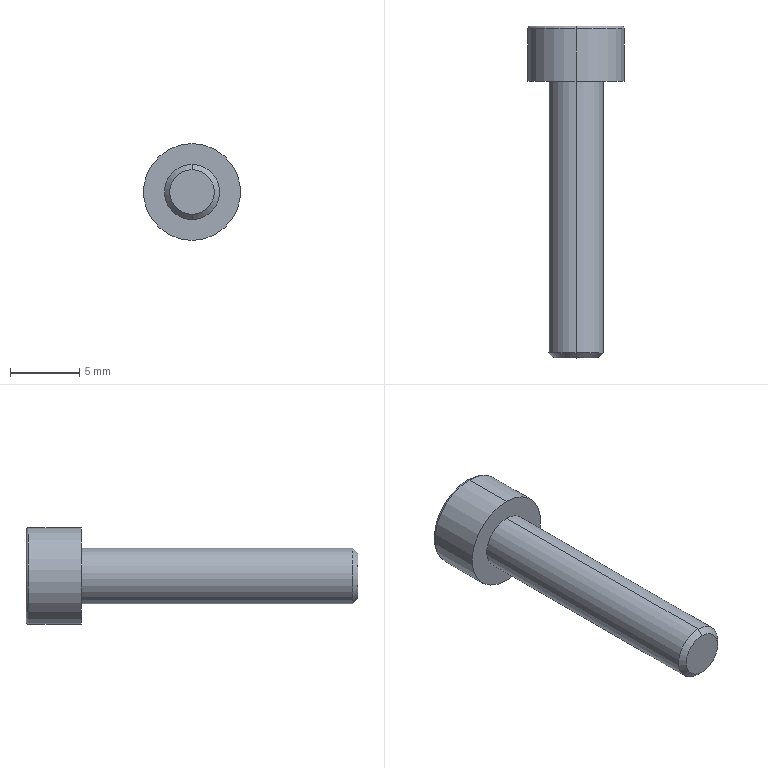Part | SolidWorks | features ICE 2, Chamfer 1, Extrusion 1, Fillet 1, RefAxis 1 | 1 solid | 18 faces | box 7 x 24 x 7 mm | volume 387.861 mm3 | plane 10 | cylinder 4 | cone 2 | torus 2 | commonest cylinder face diameters 4 x2 7 x2
STEP:
#1=CARTESIAN_POINT('',(0.,-20.,-1.61));
#2=VERTEX_POINT('',#1);
#3=CARTESIAN_POINT('',(0.,-20.,1.61));
#4=VERTEX_POINT('',#3);
#5=CARTESIAN_POINT('',(0.,-20.,0.));
#6=DIRECTION('',(0.,-1.,0.));
#7=DIRECTION('',(0.,0.,-1.));
#8=AXIS2_PLACEMENT_3D('',#5,#6,#7);
#9=CIRCLE('',#8,1.61);
#10=EDGE_CURVE('',#2,#4,#9,.T.);
#11=ORIENTED_EDGE('',*,*,#10,.F.);
#12=CARTESIAN_POINT('',(0.,-19.61,-2.));
#13=VERTEX_POINT('',#12);
#14=CARTESIAN_POINT('',(0.,-20.,-1.61));
#15=DIRECTION('',(0.,0.7071,-0.7071));
#16=VECTOR('',#15,1000.);
#17=LINE('',#14,#16);
#18=EDGE_CURVE('',#2,#13,#17,.T.);
#19=ORIENTED_EDGE('',*,*,#18,.T.);
#20=CARTESIAN_POINT('',(0.,-19.61,2.));
#21=VERTEX_POINT('',#20);
#22=CARTESIAN_POINT('',(0.,-19.61,0.));
#23=DIRECTION('',(0.,1.,0.));
#24=DIRECTION('',(0.,0.,-1.));
#25=AXIS2_PLACEMENT_3D('',#22,#23,#24);
#26=CIRCLE('',#25,2.);
#27=EDGE_CURVE('',#21,#13,#26,.T.);
#28=ORIENTED_EDGE('',*,*,#27,.F.);
#29=CARTESIAN_POINT('',(0.,-20.,1.61));
#30=DIRECTION('',(0.,0.7071,0.7071));
#31=VECTOR('',#30,1000.);
#32=LINE('',#29,#31);
#33=EDGE_CURVE('',#4,#21,#32,.T.);
#34=ORIENTED_EDGE('',*,*,#33,.F.);
#35=EDGE_LOOP('',(#11,#19,#28,#34));
#36=FACE_OUTER_BOUND('',#35,.T.);
#37=CARTESIAN_POINT('',(0.,-20.,0.));
#38=DIRECTION('',(0.,1.,0.));
#39=DIRECTION('',(0.,0.,1.));
#40=AXIS2_PLACEMENT_3D('',#37,#38,#39);
#41=CONICAL_SURFACE('',#40,1.61,0.7854);
#42=ADVANCED_FACE('',(#36),#41,.T.);
#43=ORIENTED_EDGE('',*,*,#27,.T.);
#44=CARTESIAN_POINT('',(0.,0.,-2.));
#45=VERTEX_POINT('',#44);
#46=CARTESIAN_POINT('',(0.,-20.,-2.));
#47=DIRECTION('',(0.,1.,0.));
#48=VECTOR('',#47,1000.);
#49=LINE('',#46,#48);
#50=EDGE_CURVE('',#13,#45,#49,.T.);
#51=ORIENTED_EDGE('',*,*,#50,.T.);
#52=CARTESIAN_POINT('',(0.,0.,2.));
#53=VERTEX_POINT('',#52);
#54=CARTESIAN_POINT('',(0.,0.,0.));
#55=DIRECTION('',(0.,-1.,0.));
#56=DIRECTION('',(0.,0.,1.));
#57=AXIS2_PLACEMENT_3D('',#54,#55,#56);
#58=CIRCLE('',#57,2.);
#59=EDGE_CURVE('',#45,#53,#58,.T.);
#60=ORIENTED_EDGE('',*,*,#59,.T.);
#61=CARTESIAN_POINT('',(0.,-20.,2.));
#62=DIRECTION('',(0.,1.,0.));
#63=VECTOR('',#62,1000.);
#64=LINE('',#61,#63);
#65=EDGE_CURVE('',#21,#53,#64,.T.);
#66=ORIENTED_EDGE('',*,*,#65,.F.);
#67=EDGE_LOOP('',(#43,#51,#60,#66));
#68=FACE_OUTER_BOUND('',#67,.T.);
#69=CARTESIAN_POINT('',(0.,-20.,0.));
#70=DIRECTION('',(0.,1.,0.));
#71=DIRECTION('',(0.,0.,1.));
#72=AXIS2_PLACEMENT_3D('',#69,#70,#71);
#73=CYLINDRICAL_SURFACE('',#72,2.);
#74=ADVANCED_FACE('',(#68),#73,.T.);
#75=CARTESIAN_POINT('',(0.,3.8,-3.5));
#76=VERTEX_POINT('',#75);
#77=CARTESIAN_POINT('',(0.,3.8,3.5));
#78=VERTEX_POINT('',#77);
#79=CARTESIAN_POINT('',(0.,3.8,0.));
#80=DIRECTION('',(0.,-1.,0.));
#81=DIRECTION('',(0.,0.,1.));
#82=AXIS2_PLACEMENT_3D('',#79,#80,#81);
#83=CIRCLE('',#82,3.5);
#84=EDGE_CURVE('',#76,#78,#83,.T.);
#85=ORIENTED_EDGE('',*,*,#84,.F.);
#86=CARTESIAN_POINT('',(0.,4.,-3.3));
#87=VERTEX_POINT('',#86);
#88=CARTESIAN_POINT('',(0.,3.8,-3.3));
#89=DIRECTION('',(1.,0.,0.));
#90=DIRECTION('',(0.,0.,-1.));
#91=AXIS2_PLACEMENT_3D('',#88,#89,#90);
#92=CIRCLE('',#91,0.2);
#93=EDGE_CURVE('',#76,#87,#92,.T.);
#94=ORIENTED_EDGE('',*,*,#93,.T.);
#95=CARTESIAN_POINT('',(0.,4.,3.3));
#96=VERTEX_POINT('',#95);
#97=CARTESIAN_POINT('',(0.,4.,0.));
#98=DIRECTION('',(0.,1.,0.));
#99=DIRECTION('',(0.,0.,1.));
#100=AXIS2_PLACEMENT_3D('',#97,#98,#99);
#101=CIRCLE('',#100,3.3);
#102=EDGE_CURVE('',#96,#87,#101,.T.);
#103=ORIENTED_EDGE('',*,*,#102,.F.);
#104=CARTESIAN_POINT('',(0.,3.8,3.3));
#105=DIRECTION('',(-1.,0.,0.));
#106=DIRECTION('',(0.,0.,1.));
#107=AXIS2_PLACEMENT_3D('',#104,#105,#106);
#108=CIRCLE('',#107,0.2);
#109=EDGE_CURVE('',#78,#96,#108,.T.);
#110=ORIENTED_EDGE('',*,*,#109,.F.);
#111=EDGE_LOOP('',(#85,#94,#103,#110));
#112=FACE_OUTER_BOUND('',#111,.T.);
#113=CARTESIAN_POINT('',(0.,3.8,0.));
#114=DIRECTION('',(0.,1.,0.));
#115=DIRECTION('',(0.,0.,1.));
#116=AXIS2_PLACEMENT_3D('',#113,#114,#115);
#117=TOROIDAL_SURFACE('',#116,3.3,0.2);
#118=ADVANCED_FACE('',(#112),#117,.T.);
#119=ORIENTED_EDGE('',*,*,#84,.T.);
#120=CARTESIAN_POINT('',(0.,0.,3.5));
#121=VERTEX_POINT('',#120);
#122=CARTESIAN_POINT('',(0.,4.,3.5));
#123=DIRECTION('',(0.,-1.,0.));
#124=VECTOR('',#123,1000.);
#125=LINE('',#122,#124);
#126=EDGE_CURVE('',#78,#121,#125,.T.);
#127=ORIENTED_EDGE('',*,*,#126,.T.);
#128=CARTESIAN_POINT('',(0.,0.,-3.5));
#129=VERTEX_POINT('',#128);
#130=CARTESIAN_POINT('',(0.,0.,0.));
#131=DIRECTION('',(0.,1.,0.));
#132=DIRECTION('',(0.,0.,1.));
#133=AXIS2_PLACEMENT_3D('',#130,#131,#132);
#134=CIRCLE('',#133,3.5);
#135=EDGE_CURVE('',#121,#129,#134,.T.);
#136=ORIENTED_EDGE('',*,*,#135,.T.);
#137=CARTESIAN_POINT('',(0.,4.,-3.5));
#138=DIRECTION('',(0.,-1.,0.));
#139=VECTOR('',#138,1000.);
#140=LINE('',#137,#139);
#141=EDGE_CURVE('',#76,#129,#140,.T.);
#142=ORIENTED_EDGE('',*,*,#141,.F.);
#143=EDGE_LOOP('',(#119,#127,#136,#142));
#144=FACE_OUTER_BOUND('',#143,.T.);
#145=CARTESIAN_POINT('',(0.,4.,0.));
#146=DIRECTION('',(0.,-1.,0.));
#147=DIRECTION('',(0.,0.,-1.));
#148=AXIS2_PLACEMENT_3D('',#145,#146,#147);
#149=CYLINDRICAL_SURFACE('',#148,3.5);
#150=ADVANCED_FACE('',(#144),#149,.T.);
#151=CARTESIAN_POINT('',(0.,0.,0.));
#152=DIRECTION('',(0.,1.,0.));
#153=DIRECTION('',(0.,0.,1.));
#154=AXIS2_PLACEMENT_3D('',#151,#152,#153);
#155=CIRCLE('',#154,3.5);
#156=EDGE_CURVE('',#129,#121,#155,.T.);
#157=ORIENTED_EDGE('',*,*,#156,.F.);
#158=ORIENTED_EDGE('',*,*,#135,.F.);
#159=EDGE_LOOP('',(#157,#158));
#160=FACE_OUTER_BOUND('',#159,.T.);
#161=CARTESIAN_POINT('',(0.,0.,0.));
#162=DIRECTION('',(0.,-1.,0.));
#163=DIRECTION('',(0.,0.,1.));
#164=AXIS2_PLACEMENT_3D('',#161,#162,#163);
#165=CIRCLE('',#164,2.);
#166=EDGE_CURVE('',#53,#45,#165,.T.);
#167=ORIENTED_EDGE('',*,*,#166,.F.);
#168=ORIENTED_EDGE('',*,*,#59,.F.);
#169=EDGE_LOOP('',(#167,#168));
#170=FACE_BOUND('',#169,.T.);
#171=CARTESIAN_POINT('',(0.,0.,0.));
#172=DIRECTION('',(0.,1.,0.));
#173=DIRECTION('',(0.,0.,1.));
#174=AXIS2_PLACEMENT_3D('',#171,#172,#173);
#175=PLANE('',#174);
#176=ADVANCED_FACE('',(#160,#170),#175,.F.);
#177=ORIENTED_EDGE('',*,*,#126,.F.);
#178=CARTESIAN_POINT('',(0.,3.8,0.));
#179=DIRECTION('',(0.,-1.,0.));
#180=DIRECTION('',(0.,0.,1.));
#181=AXIS2_PLACEMENT_3D('',#178,#179,#180);
#182=CIRCLE('',#181,3.5);
#183=EDGE_CURVE('',#78,#76,#182,.T.);
#184=ORIENTED_EDGE('',*,*,#183,.T.);
#185=ORIENTED_EDGE('',*,*,#141,.T.);
#186=ORIENTED_EDGE('',*,*,#156,.T.);
#187=EDGE_LOOP('',(#177,#184,#185,#186));
#188=FACE_OUTER_BOUND('',#187,.T.);
#189=CARTESIAN_POINT('',(0.,4.,0.));
#190=DIRECTION('',(0.,-1.,0.));
#191=DIRECTION('',(0.,0.,-1.));
#192=AXIS2_PLACEMENT_3D('',#189,#190,#191);
#193=CYLINDRICAL_SURFACE('',#192,3.5);
#194=ADVANCED_FACE('',(#188),#193,.T.);
#195=ORIENTED_EDGE('',*,*,#102,.T.);
#196=CARTESIAN_POINT('',(0.,4.,0.));
#197=DIRECTION('',(0.,1.,0.));
#198=DIRECTION('',(0.,0.,1.));
#199=AXIS2_PLACEMENT_3D('',#196,#197,#198);
#200=CIRCLE('',#199,3.3);
#201=EDGE_CURVE('',#87,#96,#200,.T.);
#202=ORIENTED_EDGE('',*,*,#201,.T.);
#203=EDGE_LOOP('',(#195,#202));
#204=FACE_OUTER_BOUND('',#203,.T.);
#205=CARTESIAN_POINT('',(0.8862,4.,1.535));
#206=VERTEX_POINT('',#205);
#207=CARTESIAN_POINT('',(1.772,4.,0.));
#208=VERTEX_POINT('',#207);
#209=CARTESIAN_POINT('',(0.8862,4.,1.535));
#210=DIRECTION('',(0.5,0.,-0.866));
#211=VECTOR('',#210,1000.);
#212=LINE('',#209,#211);
#213=EDGE_CURVE('',#206,#208,#212,.T.);
#214=ORIENTED_EDGE('',*,*,#213,.F.);
#215=CARTESIAN_POINT('',(-0.8862,4.,1.535));
#216=VERTEX_POINT('',#215);
#217=CARTESIAN_POINT('',(-0.8862,4.,1.535));
#218=DIRECTION('',(1.,0.,0.));
#219=VECTOR('',#218,1000.);
#220=LINE('',#217,#219);
#221=EDGE_CURVE('',#216,#206,#220,.T.);
#222=ORIENTED_EDGE('',*,*,#221,.F.);
#223=CARTESIAN_POINT('',(-1.772,4.,0.));
#224=VERTEX_POINT('',#223);
#225=CARTESIAN_POINT('',(-1.772,4.,0.));
#226=DIRECTION('',(0.5,0.,0.866));
#227=VECTOR('',#226,1000.);
#228=LINE('',#225,#227);
#229=EDGE_CURVE('',#224,#216,#228,.T.);
#230=ORIENTED_EDGE('',*,*,#229,.F.);
#231=CARTESIAN_POINT('',(-0.8862,4.,-1.535));
#232=VERTEX_POINT('',#231);
#233=CARTESIAN_POINT('',(-0.8862,4.,-1.535));
#234=DIRECTION('',(-0.5,0.,0.866));
#235=VECTOR('',#234,1000.);
#236=LINE('',#233,#235);
#237=EDGE_CURVE('',#232,#224,#236,.T.);
#238=ORIENTED_EDGE('',*,*,#237,.F.);
#239=CARTESIAN_POINT('',(0.8862,4.,-1.535));
#240=VERTEX_POINT('',#239);
#241=CARTESIAN_POINT('',(0.8862,4.,-1.535));
#242=DIRECTION('',(-1.,0.,0.));
#243=VECTOR('',#242,1000.);
#244=LINE('',#241,#243);
#245=EDGE_CURVE('',#240,#232,#244,.T.);
#246=ORIENTED_EDGE('',*,*,#245,.F.);
#247=CARTESIAN_POINT('',(1.772,4.,0.));
#248=DIRECTION('',(-0.5,0.,-0.866));
#249=VECTOR('',#248,1000.);
#250=LINE('',#247,#249);
#251=EDGE_CURVE('',#208,#240,#250,.T.);
#252=ORIENTED_EDGE('',*,*,#251,.F.);
#253=EDGE_LOOP('',(#214,#222,#230,#238,#246,#252));
#254=FACE_BOUND('',#253,.T.);
#255=CARTESIAN_POINT('',(0.,4.,0.));
#256=DIRECTION('',(0.,1.,0.));
#257=DIRECTION('',(0.,0.,1.));
#258=AXIS2_PLACEMENT_3D('',#255,#256,#257);
#259=PLANE('',#258);
#260=ADVANCED_FACE('',(#204,#254),#259,.T.);
#261=ORIENTED_EDGE('',*,*,#213,.T.);
#262=CARTESIAN_POINT('',(1.772,2.,0.));
#263=VERTEX_POINT('',#262);
#264=CARTESIAN_POINT('',(1.772,2.,0.));
#265=DIRECTION('',(0.,1.,0.));
#266=VECTOR('',#265,1000.);
#267=LINE('',#264,#266);
#268=EDGE_CURVE('',#263,#208,#267,.T.);
#269=ORIENTED_EDGE('',*,*,#268,.F.);
#270=CARTESIAN_POINT('',(0.8862,2.,1.535));
#271=VERTEX_POINT('',#270);
#272=CARTESIAN_POINT('',(0.8862,2.,1.535));
#273=DIRECTION('',(0.5,0.,-0.866));
#274=VECTOR('',#273,1000.);
#275=LINE('',#272,#274);
#276=EDGE_CURVE('',#271,#263,#275,.T.);
#277=ORIENTED_EDGE('',*,*,#276,.F.);
#278=CARTESIAN_POINT('',(0.8862,2.,1.535));
#279=DIRECTION('',(0.,1.,0.));
#280=VECTOR('',#279,1000.);
#281=LINE('',#278,#280);
#282=EDGE_CURVE('',#271,#206,#281,.T.);
#283=ORIENTED_EDGE('',*,*,#282,.T.);
#284=EDGE_LOOP('',(#261,#269,#277,#283));
#285=FACE_OUTER_BOUND('',#284,.T.);
#286=CARTESIAN_POINT('',(0.8862,2.,1.535));
#287=DIRECTION('',(0.866,0.,0.5));
#288=DIRECTION('',(0.5,0.,-0.866));
#289=AXIS2_PLACEMENT_3D('',#286,#287,#288);
#290=PLANE('',#289);
#291=ADVANCED_FACE('',(#285),#290,.F.);
#292=ORIENTED_EDGE('',*,*,#221,.T.);
#293=ORIENTED_EDGE('',*,*,#282,.F.);
#294=CARTESIAN_POINT('',(-0.8862,2.,1.535));
#295=VERTEX_POINT('',#294);
#296=CARTESIAN_POINT('',(-0.8862,2.,1.535));
#297=DIRECTION('',(1.,0.,0.));
#298=VECTOR('',#297,1000.);
#299=LINE('',#296,#298);
#300=EDGE_CURVE('',#295,#271,#299,.T.);
#301=ORIENTED_EDGE('',*,*,#300,.F.);
#302=CARTESIAN_POINT('',(-0.8862,2.,1.535));
#303=DIRECTION('',(0.,1.,0.));
#304=VECTOR('',#303,1000.);
#305=LINE('',#302,#304);
#306=EDGE_CURVE('',#295,#216,#305,.T.);
#307=ORIENTED_EDGE('',*,*,#306,.T.);
#308=EDGE_LOOP('',(#292,#293,#301,#307));
#309=FACE_OUTER_BOUND('',#308,.T.);
#310=CARTESIAN_POINT('',(-0.8862,2.,1.535));
#311=DIRECTION('',(0.,0.,1.));
#312=DIRECTION('',(1.,0.,0.));
#313=AXIS2_PLACEMENT_3D('',#310,#311,#312);
#314=PLANE('',#313);
#315=ADVANCED_FACE('',(#309),#314,.F.);
#316=ORIENTED_EDGE('',*,*,#229,.T.);
#317=ORIENTED_EDGE('',*,*,#306,.F.);
#318=CARTESIAN_POINT('',(-1.772,2.,0.));
#319=VERTEX_POINT('',#318);
#320=CARTESIAN_POINT('',(-1.772,2.,0.));
#321=DIRECTION('',(0.5,0.,0.866));
#322=VECTOR('',#321,1000.);
#323=LINE('',#320,#322);
#324=EDGE_CURVE('',#319,#295,#323,.T.);
#325=ORIENTED_EDGE('',*,*,#324,.F.);
#326=CARTESIAN_POINT('',(-1.772,2.,0.));
#327=DIRECTION('',(0.,1.,0.));
#328=VECTOR('',#327,1000.);
#329=LINE('',#326,#328);
#330=EDGE_CURVE('',#319,#224,#329,.T.);
#331=ORIENTED_EDGE('',*,*,#330,.T.);
#332=EDGE_LOOP('',(#316,#317,#325,#331));
#333=FACE_OUTER_BOUND('',#332,.T.);
#334=CARTESIAN_POINT('',(-1.772,2.,0.));
#335=DIRECTION('',(-0.866,0.,0.5));
#336=DIRECTION('',(0.5,0.,0.866));
#337=AXIS2_PLACEMENT_3D('',#334,#335,#336);
#338=PLANE('',#337);
#339=ADVANCED_FACE('',(#333),#338,.F.);
#340=ORIENTED_EDGE('',*,*,#237,.T.);
#341=ORIENTED_EDGE('',*,*,#330,.F.);
#342=CARTESIAN_POINT('',(-0.8862,2.,-1.535));
#343=VERTEX_POINT('',#342);
#344=CARTESIAN_POINT('',(-0.8862,2.,-1.535));
#345=DIRECTION('',(-0.5,0.,0.866));
#346=VECTOR('',#345,1000.);
#347=LINE('',#344,#346);
#348=EDGE_CURVE('',#343,#319,#347,.T.);
#349=ORIENTED_EDGE('',*,*,#348,.F.);
#350=CARTESIAN_POINT('',(-0.8862,2.,-1.535));
#351=DIRECTION('',(0.,1.,0.));
#352=VECTOR('',#351,1000.);
#353=LINE('',#350,#352);
#354=EDGE_CURVE('',#343,#232,#353,.T.);
#355=ORIENTED_EDGE('',*,*,#354,.T.);
#356=EDGE_LOOP('',(#340,#341,#349,#355));
#357=FACE_OUTER_BOUND('',#356,.T.);
#358=CARTESIAN_POINT('',(-0.8862,2.,-1.535));
#359=DIRECTION('',(-0.866,0.,-0.5));
#360=DIRECTION('',(-0.5,0.,0.866));
#361=AXIS2_PLACEMENT_3D('',#358,#359,#360);
#362=PLANE('',#361);
#363=ADVANCED_FACE('',(#357),#362,.F.);
#364=ORIENTED_EDGE('',*,*,#245,.T.);
#365=ORIENTED_EDGE('',*,*,#354,.F.);
#366=CARTESIAN_POINT('',(0.8862,2.,-1.535));
#367=VERTEX_POINT('',#366);
#368=CARTESIAN_POINT('',(0.8862,2.,-1.535));
#369=DIRECTION('',(-1.,0.,0.));
#370=VECTOR('',#369,1000.);
#371=LINE('',#368,#370);
#372=EDGE_CURVE('',#367,#343,#371,.T.);
#373=ORIENTED_EDGE('',*,*,#372,.F.);
#374=CARTESIAN_POINT('',(0.8862,2.,-1.535));
#375=DIRECTION('',(0.,1.,0.));
#376=VECTOR('',#375,1000.);
#377=LINE('',#374,#376);
#378=EDGE_CURVE('',#367,#240,#377,.T.);
#379=ORIENTED_EDGE('',*,*,#378,.T.);
#380=EDGE_LOOP('',(#364,#365,#373,#379));
#381=FACE_OUTER_BOUND('',#380,.T.);
#382=CARTESIAN_POINT('',(0.8862,2.,-1.535));
#383=DIRECTION('',(0.,0.,-1.));
#384=DIRECTION('',(-1.,0.,0.));
#385=AXIS2_PLACEMENT_3D('',#382,#383,#384);
#386=PLANE('',#385);
#387=ADVANCED_FACE('',(#381),#386,.F.);
#388=ORIENTED_EDGE('',*,*,#251,.T.);
#389=ORIENTED_EDGE('',*,*,#378,.F.);
#390=CARTESIAN_POINT('',(1.772,2.,0.));
#391=DIRECTION('',(-0.5,0.,-0.866));
#392=VECTOR('',#391,1000.);
#393=LINE('',#390,#392);
#394=EDGE_CURVE('',#263,#367,#393,.T.);
#395=ORIENTED_EDGE('',*,*,#394,.F.);
#396=ORIENTED_EDGE('',*,*,#268,.T.);
#397=EDGE_LOOP('',(#388,#389,#395,#396));
#398=FACE_OUTER_BOUND('',#397,.T.);
#399=CARTESIAN_POINT('',(1.772,2.,0.));
#400=DIRECTION('',(0.866,0.,-0.5));
#401=DIRECTION('',(-0.5,0.,-0.866));
#402=AXIS2_PLACEMENT_3D('',#399,#400,#401);
#403=PLANE('',#402);
#404=ADVANCED_FACE('',(#398),#403,.F.);
#405=ORIENTED_EDGE('',*,*,#276,.T.);
#406=ORIENTED_EDGE('',*,*,#394,.T.);
#407=ORIENTED_EDGE('',*,*,#372,.T.);
#408=ORIENTED_EDGE('',*,*,#348,.T.);
#409=ORIENTED_EDGE('',*,*,#324,.T.);
#410=ORIENTED_EDGE('',*,*,#300,.T.);
#411=EDGE_LOOP('',(#405,#406,#407,#408,#409,#410));
#412=FACE_OUTER_BOUND('',#411,.T.);
#413=CARTESIAN_POINT('',(0.,2.,0.));
#414=DIRECTION('',(0.,1.,0.));
#415=DIRECTION('',(0.,0.,1.));
#416=AXIS2_PLACEMENT_3D('',#413,#414,#415);
#417=PLANE('',#416);
#418=ADVANCED_FACE('',(#412),#417,.T.);
#419=ORIENTED_EDGE('',*,*,#93,.F.);
#420=ORIENTED_EDGE('',*,*,#183,.F.);
#421=ORIENTED_EDGE('',*,*,#109,.T.);
#422=ORIENTED_EDGE('',*,*,#201,.F.);
#423=EDGE_LOOP('',(#419,#420,#421,#422));
#424=FACE_OUTER_BOUND('',#423,.T.);
#425=CARTESIAN_POINT('',(0.,3.8,0.));
#426=DIRECTION('',(0.,1.,0.));
#427=DIRECTION('',(0.,0.,1.));
#428=AXIS2_PLACEMENT_3D('',#425,#426,#427);
#429=TOROIDAL_SURFACE('',#428,3.3,0.2);
#430=ADVANCED_FACE('',(#424),#429,.T.);
#431=ORIENTED_EDGE('',*,*,#50,.F.);
#432=CARTESIAN_POINT('',(0.,-19.61,0.));
#433=DIRECTION('',(0.,1.,0.));
#434=DIRECTION('',(0.,0.,-1.));
#435=AXIS2_PLACEMENT_3D('',#432,#433,#434);
#436=CIRCLE('',#435,2.);
#437=EDGE_CURVE('',#13,#21,#436,.T.);
#438=ORIENTED_EDGE('',*,*,#437,.T.);
#439=ORIENTED_EDGE('',*,*,#65,.T.);
#440=ORIENTED_EDGE('',*,*,#166,.T.);
#441=EDGE_LOOP('',(#431,#438,#439,#440));
#442=FACE_OUTER_BOUND('',#441,.T.);
#443=CARTESIAN_POINT('',(0.,-20.,0.));
#444=DIRECTION('',(0.,1.,0.));
#445=DIRECTION('',(0.,0.,1.));
#446=AXIS2_PLACEMENT_3D('',#443,#444,#445);
#447=CYLINDRICAL_SURFACE('',#446,2.);
#448=ADVANCED_FACE('',(#442),#447,.T.);
#449=CARTESIAN_POINT('',(0.,-20.,0.));
#450=DIRECTION('',(0.,-1.,0.));
#451=DIRECTION('',(0.,0.,-1.));
#452=AXIS2_PLACEMENT_3D('',#449,#450,#451);
#453=CIRCLE('',#452,1.61);
#454=EDGE_CURVE('',#4,#2,#453,.T.);
#455=ORIENTED_EDGE('',*,*,#454,.T.);
#456=ORIENTED_EDGE('',*,*,#10,.T.);
#457=EDGE_LOOP('',(#455,#456));
#458=FACE_OUTER_BOUND('',#457,.T.);
#459=CARTESIAN_POINT('',(0.,-20.,0.));
#460=DIRECTION('',(0.,-1.,0.));
#461=DIRECTION('',(0.,0.,-1.));
#462=AXIS2_PLACEMENT_3D('',#459,#460,#461);
#463=PLANE('',#462);
#464=ADVANCED_FACE('',(#458),#463,.T.);
#465=ORIENTED_EDGE('',*,*,#18,.F.);
#466=ORIENTED_EDGE('',*,*,#454,.F.);
#467=ORIENTED_EDGE('',*,*,#33,.T.);
#468=ORIENTED_EDGE('',*,*,#437,.F.);
#469=EDGE_LOOP('',(#465,#466,#467,#468));
#470=FACE_OUTER_BOUND('',#469,.T.);
#471=CARTESIAN_POINT('',(0.,-20.,0.));
#472=DIRECTION('',(0.,1.,0.));
#473=DIRECTION('',(0.,0.,1.));
#474=AXIS2_PLACEMENT_3D('',#471,#472,#473);
#475=CONICAL_SURFACE('',#474,1.61,0.7854);
#476=ADVANCED_FACE('',(#470),#475,.T.);
#477=CLOSED_SHELL('',(#42,#74,#118,#150,#176,#194,#260,#291,#315,#339,#363,#387,#404,#418,#430,#448,#464,#476));
#478=MANIFOLD_SOLID_BREP('',#477);
#479=CARTESIAN_POINT('',(0.,0.,0.));
#480=DIRECTION('',(0.,0.,1.));
#481=DIRECTION('',(1.,0.,0.));
#482=AXIS2_PLACEMENT_3D('',#479,#480,#481);
#483=(LENGTH_UNIT()NAMED_UNIT(*)SI_UNIT(.MILLI.,.METRE.));
#484=UNCERTAINTY_MEASURE_WITH_UNIT(LENGTH_MEASURE(0.00001),#483,'','');
#485=(NAMED_UNIT(*)PLANE_ANGLE_UNIT()SI_UNIT($,.RADIAN.));
#486=(NAMED_UNIT(*)SI_UNIT($,.STERADIAN.)SOLID_ANGLE_UNIT());
#487=(GEOMETRIC_REPRESENTATION_CONTEXT(3)GLOBAL_UNCERTAINTY_ASSIGNED_CONTEXT((#484))GLOBAL_UNIT_ASSIGNED_CONTEXT((#483,#485,#486))REPRESENTATION_CONTEXT('',''));
#488=ADVANCED_BREP_SHAPE_REPRESENTATION('',(#478,#482),#487);